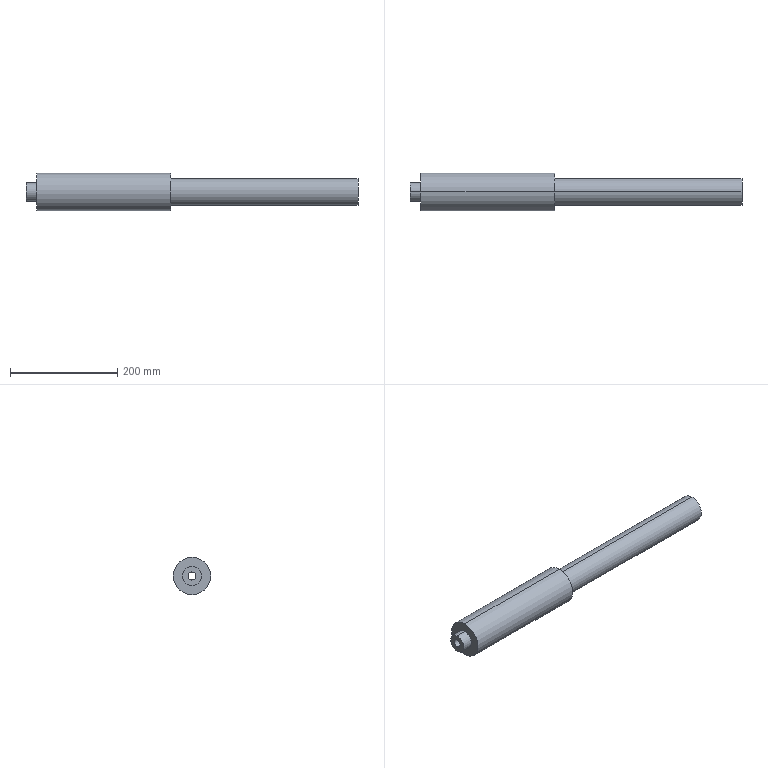Part | SolidWorks | features Revolution 1 | 1 solid | 18 faces | box 620 x 70 x 70 mm | volume 957204 mm3 | cylinder 12 | plane 6 | commonest cylinder face diameters 50 x4 15 x2 30 x2 35 x2 70 x2
STEP:
#1=CARTESIAN_POINT('',(271.174,193.285,-25.));
#2=VERTEX_POINT('',#1);
#3=CARTESIAN_POINT('',(271.174,193.285,25.));
#4=VERTEX_POINT('',#3);
#5=CARTESIAN_POINT('',(271.174,193.285,0.));
#6=DIRECTION('',(-1.,0.,0.));
#7=DIRECTION('',(0.,0.,1.));
#8=AXIS2_PLACEMENT_3D('',#5,#6,#7);
#9=CIRCLE('',#8,25.);
#10=EDGE_CURVE('',#2,#4,#9,.T.);
#11=ORIENTED_EDGE('',*,*,#10,.F.);
#12=CARTESIAN_POINT('',(41.174,193.285,-25.));
#13=VERTEX_POINT('',#12);
#14=CARTESIAN_POINT('',(-12.561,193.285,-25.));
#15=DIRECTION('',(-1.,0.,0.));
#16=VECTOR('',#15,1000.);
#17=LINE('',#14,#16);
#18=EDGE_CURVE('',#2,#13,#17,.T.);
#19=ORIENTED_EDGE('',*,*,#18,.T.);
#20=CARTESIAN_POINT('',(41.174,193.285,25.));
#21=VERTEX_POINT('',#20);
#22=CARTESIAN_POINT('',(41.174,193.285,0.));
#23=DIRECTION('',(-1.,0.,0.));
#24=DIRECTION('',(0.,0.,1.));
#25=AXIS2_PLACEMENT_3D('',#22,#23,#24);
#26=CIRCLE('',#25,25.);
#27=EDGE_CURVE('',#13,#21,#26,.T.);
#28=ORIENTED_EDGE('',*,*,#27,.T.);
#29=CARTESIAN_POINT('',(-12.561,193.285,25.));
#30=DIRECTION('',(-1.,0.,0.));
#31=VECTOR('',#30,1000.);
#32=LINE('',#29,#31);
#33=EDGE_CURVE('',#4,#21,#32,.T.);
#34=ORIENTED_EDGE('',*,*,#33,.F.);
#35=EDGE_LOOP('',(#11,#19,#28,#34));
#36=FACE_OUTER_BOUND('',#35,.T.);
#37=CARTESIAN_POINT('',(-12.561,193.285,0.));
#38=DIRECTION('',(-1.,0.,0.));
#39=DIRECTION('',(0.,0.,1.));
#40=AXIS2_PLACEMENT_3D('',#37,#38,#39);
#41=CYLINDRICAL_SURFACE('',#40,25.);
#42=ADVANCED_FACE('',(#36),#41,.F.);
#43=CARTESIAN_POINT('',(41.174,193.285,-7.5));
#44=VERTEX_POINT('',#43);
#45=CARTESIAN_POINT('',(41.174,193.285,7.5));
#46=VERTEX_POINT('',#45);
#47=CARTESIAN_POINT('',(41.174,193.285,0.));
#48=DIRECTION('',(-1.,0.,0.));
#49=DIRECTION('',(0.,0.,1.));
#50=AXIS2_PLACEMENT_3D('',#47,#48,#49);
#51=CIRCLE('',#50,7.5);
#52=EDGE_CURVE('',#44,#46,#51,.T.);
#53=ORIENTED_EDGE('',*,*,#52,.F.);
#54=CARTESIAN_POINT('',(11.174,193.285,-7.5));
#55=VERTEX_POINT('',#54);
#56=CARTESIAN_POINT('',(-12.561,193.285,-7.5));
#57=DIRECTION('',(-1.,0.,0.));
#58=VECTOR('',#57,1000.);
#59=LINE('',#56,#58);
#60=EDGE_CURVE('',#44,#55,#59,.T.);
#61=ORIENTED_EDGE('',*,*,#60,.T.);
#62=CARTESIAN_POINT('',(11.174,193.285,7.5));
#63=VERTEX_POINT('',#62);
#64=CARTESIAN_POINT('',(11.174,193.285,0.));
#65=DIRECTION('',(-1.,0.,0.));
#66=DIRECTION('',(0.,0.,1.));
#67=AXIS2_PLACEMENT_3D('',#64,#65,#66);
#68=CIRCLE('',#67,7.5);
#69=EDGE_CURVE('',#55,#63,#68,.T.);
#70=ORIENTED_EDGE('',*,*,#69,.T.);
#71=CARTESIAN_POINT('',(-12.561,193.285,7.5));
#72=DIRECTION('',(-1.,0.,0.));
#73=VECTOR('',#72,1000.);
#74=LINE('',#71,#73);
#75=EDGE_CURVE('',#46,#63,#74,.T.);
#76=ORIENTED_EDGE('',*,*,#75,.F.);
#77=EDGE_LOOP('',(#53,#61,#70,#76));
#78=FACE_OUTER_BOUND('',#77,.T.);
#79=CARTESIAN_POINT('',(-12.561,193.285,0.));
#80=DIRECTION('',(-1.,0.,0.));
#81=DIRECTION('',(0.,0.,1.));
#82=AXIS2_PLACEMENT_3D('',#79,#80,#81);
#83=CYLINDRICAL_SURFACE('',#82,7.5);
#84=ADVANCED_FACE('',(#78),#83,.F.);
#85=CARTESIAN_POINT('',(31.174,193.285,17.5));
#86=VERTEX_POINT('',#85);
#87=CARTESIAN_POINT('',(31.174,193.285,-17.5));
#88=VERTEX_POINT('',#87);
#89=CARTESIAN_POINT('',(31.174,193.285,0.));
#90=DIRECTION('',(-1.,0.,0.));
#91=DIRECTION('',(0.,0.,1.));
#92=AXIS2_PLACEMENT_3D('',#89,#90,#91);
#93=CIRCLE('',#92,17.5);
#94=EDGE_CURVE('',#86,#88,#93,.T.);
#95=ORIENTED_EDGE('',*,*,#94,.T.);
#96=CARTESIAN_POINT('',(11.174,193.285,-17.5));
#97=VERTEX_POINT('',#96);
#98=CARTESIAN_POINT('',(-12.561,193.285,-17.5));
#99=DIRECTION('',(-1.,0.,0.));
#100=VECTOR('',#99,1000.);
#101=LINE('',#98,#100);
#102=EDGE_CURVE('',#88,#97,#101,.T.);
#103=ORIENTED_EDGE('',*,*,#102,.T.);
#104=CARTESIAN_POINT('',(11.174,193.285,17.5));
#105=VERTEX_POINT('',#104);
#106=CARTESIAN_POINT('',(11.174,193.285,0.));
#107=DIRECTION('',(-1.,0.,0.));
#108=DIRECTION('',(0.,0.,1.));
#109=AXIS2_PLACEMENT_3D('',#106,#107,#108);
#110=CIRCLE('',#109,17.5);
#111=EDGE_CURVE('',#105,#97,#110,.T.);
#112=ORIENTED_EDGE('',*,*,#111,.F.);
#113=CARTESIAN_POINT('',(-12.561,193.285,17.5));
#114=DIRECTION('',(-1.,0.,0.));
#115=VECTOR('',#114,1000.);
#116=LINE('',#113,#115);
#117=EDGE_CURVE('',#86,#105,#116,.T.);
#118=ORIENTED_EDGE('',*,*,#117,.F.);
#119=EDGE_LOOP('',(#95,#103,#112,#118));
#120=FACE_OUTER_BOUND('',#119,.T.);
#121=CARTESIAN_POINT('',(-12.561,193.285,0.));
#122=DIRECTION('',(-1.,0.,0.));
#123=DIRECTION('',(0.,0.,1.));
#124=AXIS2_PLACEMENT_3D('',#121,#122,#123);
#125=CYLINDRICAL_SURFACE('',#124,17.5);
#126=ADVANCED_FACE('',(#120),#125,.T.);
#127=CARTESIAN_POINT('',(281.174,193.285,35.));
#128=VERTEX_POINT('',#127);
#129=CARTESIAN_POINT('',(281.174,193.285,-35.));
#130=VERTEX_POINT('',#129);
#131=CARTESIAN_POINT('',(281.174,193.285,0.));
#132=DIRECTION('',(-1.,0.,0.));
#133=DIRECTION('',(0.,0.,1.));
#134=AXIS2_PLACEMENT_3D('',#131,#132,#133);
#135=CIRCLE('',#134,35.);
#136=EDGE_CURVE('',#128,#130,#135,.T.);
#137=ORIENTED_EDGE('',*,*,#136,.T.);
#138=CARTESIAN_POINT('',(31.174,193.285,-35.));
#139=VERTEX_POINT('',#138);
#140=CARTESIAN_POINT('',(-12.561,193.285,-35.));
#141=DIRECTION('',(-1.,0.,0.));
#142=VECTOR('',#141,1000.);
#143=LINE('',#140,#142);
#144=EDGE_CURVE('',#130,#139,#143,.T.);
#145=ORIENTED_EDGE('',*,*,#144,.T.);
#146=CARTESIAN_POINT('',(31.174,193.285,35.));
#147=VERTEX_POINT('',#146);
#148=CARTESIAN_POINT('',(31.174,193.285,0.));
#149=DIRECTION('',(-1.,0.,0.));
#150=DIRECTION('',(0.,0.,1.));
#151=AXIS2_PLACEMENT_3D('',#148,#149,#150);
#152=CIRCLE('',#151,35.);
#153=EDGE_CURVE('',#147,#139,#152,.T.);
#154=ORIENTED_EDGE('',*,*,#153,.F.);
#155=CARTESIAN_POINT('',(-12.561,193.285,35.));
#156=DIRECTION('',(-1.,0.,0.));
#157=VECTOR('',#156,1000.);
#158=LINE('',#155,#157);
#159=EDGE_CURVE('',#128,#147,#158,.T.);
#160=ORIENTED_EDGE('',*,*,#159,.F.);
#161=EDGE_LOOP('',(#137,#145,#154,#160));
#162=FACE_OUTER_BOUND('',#161,.T.);
#163=CARTESIAN_POINT('',(-12.561,193.285,0.));
#164=DIRECTION('',(-1.,0.,0.));
#165=DIRECTION('',(0.,0.,1.));
#166=AXIS2_PLACEMENT_3D('',#163,#164,#165);
#167=CYLINDRICAL_SURFACE('',#166,35.);
#168=ADVANCED_FACE('',(#162),#167,.T.);
#169=CARTESIAN_POINT('',(631.174,193.285,25.));
#170=VERTEX_POINT('',#169);
#171=CARTESIAN_POINT('',(631.174,193.285,-25.));
#172=VERTEX_POINT('',#171);
#173=CARTESIAN_POINT('',(631.174,193.285,0.));
#174=DIRECTION('',(-1.,0.,0.));
#175=DIRECTION('',(0.,0.,1.));
#176=AXIS2_PLACEMENT_3D('',#173,#174,#175);
#177=CIRCLE('',#176,25.);
#178=EDGE_CURVE('',#170,#172,#177,.T.);
#179=ORIENTED_EDGE('',*,*,#178,.T.);
#180=CARTESIAN_POINT('',(281.174,193.285,-25.));
#181=VERTEX_POINT('',#180);
#182=CARTESIAN_POINT('',(-12.561,193.285,-25.));
#183=DIRECTION('',(-1.,0.,0.));
#184=VECTOR('',#183,1000.);
#185=LINE('',#182,#184);
#186=EDGE_CURVE('',#172,#181,#185,.T.);
#187=ORIENTED_EDGE('',*,*,#186,.T.);
#188=CARTESIAN_POINT('',(281.174,193.285,25.));
#189=VERTEX_POINT('',#188);
#190=CARTESIAN_POINT('',(281.174,193.285,0.));
#191=DIRECTION('',(-1.,0.,0.));
#192=DIRECTION('',(0.,0.,1.));
#193=AXIS2_PLACEMENT_3D('',#190,#191,#192);
#194=CIRCLE('',#193,25.);
#195=EDGE_CURVE('',#189,#181,#194,.T.);
#196=ORIENTED_EDGE('',*,*,#195,.F.);
#197=CARTESIAN_POINT('',(-12.561,193.285,25.));
#198=DIRECTION('',(-1.,0.,0.));
#199=VECTOR('',#198,1000.);
#200=LINE('',#197,#199);
#201=EDGE_CURVE('',#170,#189,#200,.T.);
#202=ORIENTED_EDGE('',*,*,#201,.F.);
#203=EDGE_LOOP('',(#179,#187,#196,#202));
#204=FACE_OUTER_BOUND('',#203,.T.);
#205=CARTESIAN_POINT('',(-12.561,193.285,0.));
#206=DIRECTION('',(-1.,0.,0.));
#207=DIRECTION('',(0.,0.,1.));
#208=AXIS2_PLACEMENT_3D('',#205,#206,#207);
#209=CYLINDRICAL_SURFACE('',#208,25.);
#210=ADVANCED_FACE('',(#204),#209,.T.);
#211=CARTESIAN_POINT('',(631.174,193.285,-15.));
#212=VERTEX_POINT('',#211);
#213=CARTESIAN_POINT('',(631.174,193.285,15.));
#214=VERTEX_POINT('',#213);
#215=CARTESIAN_POINT('',(631.174,193.285,0.));
#216=DIRECTION('',(-1.,0.,0.));
#217=DIRECTION('',(0.,0.,1.));
#218=AXIS2_PLACEMENT_3D('',#215,#216,#217);
#219=CIRCLE('',#218,15.);
#220=EDGE_CURVE('',#212,#214,#219,.T.);
#221=ORIENTED_EDGE('',*,*,#220,.F.);
#222=CARTESIAN_POINT('',(271.174,193.285,-15.));
#223=VERTEX_POINT('',#222);
#224=CARTESIAN_POINT('',(-12.561,193.285,-15.));
#225=DIRECTION('',(-1.,0.,0.));
#226=VECTOR('',#225,1000.);
#227=LINE('',#224,#226);
#228=EDGE_CURVE('',#212,#223,#227,.T.);
#229=ORIENTED_EDGE('',*,*,#228,.T.);
#230=CARTESIAN_POINT('',(271.174,193.285,15.));
#231=VERTEX_POINT('',#230);
#232=CARTESIAN_POINT('',(271.174,193.285,0.));
#233=DIRECTION('',(-1.,0.,0.));
#234=DIRECTION('',(0.,0.,1.));
#235=AXIS2_PLACEMENT_3D('',#232,#233,#234);
#236=CIRCLE('',#235,15.);
#237=EDGE_CURVE('',#223,#231,#236,.T.);
#238=ORIENTED_EDGE('',*,*,#237,.T.);
#239=CARTESIAN_POINT('',(-12.561,193.285,15.));
#240=DIRECTION('',(-1.,0.,0.));
#241=VECTOR('',#240,1000.);
#242=LINE('',#239,#241);
#243=EDGE_CURVE('',#214,#231,#242,.T.);
#244=ORIENTED_EDGE('',*,*,#243,.F.);
#245=EDGE_LOOP('',(#221,#229,#238,#244));
#246=FACE_OUTER_BOUND('',#245,.T.);
#247=CARTESIAN_POINT('',(-12.561,193.285,0.));
#248=DIRECTION('',(-1.,0.,0.));
#249=DIRECTION('',(0.,0.,1.));
#250=AXIS2_PLACEMENT_3D('',#247,#248,#249);
#251=CYLINDRICAL_SURFACE('',#250,15.);
#252=ADVANCED_FACE('',(#246),#251,.F.);
#253=ORIENTED_EDGE('',*,*,#228,.F.);
#254=CARTESIAN_POINT('',(631.174,193.285,0.));
#255=DIRECTION('',(-1.,0.,0.));
#256=DIRECTION('',(0.,0.,1.));
#257=AXIS2_PLACEMENT_3D('',#254,#255,#256);
#258=CIRCLE('',#257,15.);
#259=EDGE_CURVE('',#214,#212,#258,.T.);
#260=ORIENTED_EDGE('',*,*,#259,.F.);
#261=ORIENTED_EDGE('',*,*,#243,.T.);
#262=CARTESIAN_POINT('',(271.174,193.285,0.));
#263=DIRECTION('',(-1.,0.,0.));
#264=DIRECTION('',(0.,0.,1.));
#265=AXIS2_PLACEMENT_3D('',#262,#263,#264);
#266=CIRCLE('',#265,15.);
#267=EDGE_CURVE('',#231,#223,#266,.T.);
#268=ORIENTED_EDGE('',*,*,#267,.T.);
#269=EDGE_LOOP('',(#253,#260,#261,#268));
#270=FACE_OUTER_BOUND('',#269,.T.);
#271=CARTESIAN_POINT('',(-12.561,193.285,0.));
#272=DIRECTION('',(-1.,0.,0.));
#273=DIRECTION('',(0.,0.,1.));
#274=AXIS2_PLACEMENT_3D('',#271,#272,#273);
#275=CYLINDRICAL_SURFACE('',#274,15.);
#276=ADVANCED_FACE('',(#270),#275,.F.);
#277=ORIENTED_EDGE('',*,*,#178,.F.);
#278=CARTESIAN_POINT('',(631.174,193.285,0.));
#279=DIRECTION('',(-1.,0.,0.));
#280=DIRECTION('',(0.,0.,1.));
#281=AXIS2_PLACEMENT_3D('',#278,#279,#280);
#282=CIRCLE('',#281,25.);
#283=EDGE_CURVE('',#172,#170,#282,.T.);
#284=ORIENTED_EDGE('',*,*,#283,.F.);
#285=EDGE_LOOP('',(#277,#284));
#286=FACE_OUTER_BOUND('',#285,.T.);
#287=ORIENTED_EDGE('',*,*,#259,.T.);
#288=ORIENTED_EDGE('',*,*,#220,.T.);
#289=EDGE_LOOP('',(#287,#288));
#290=FACE_BOUND('',#289,.T.);
#291=CARTESIAN_POINT('',(631.174,208.285,0.));
#292=DIRECTION('',(-1.,0.,0.));
#293=DIRECTION('',(0.,0.,1.));
#294=AXIS2_PLACEMENT_3D('',#291,#292,#293);
#295=PLANE('',#294);
#296=ADVANCED_FACE('',(#286,#290),#295,.F.);
#297=ORIENTED_EDGE('',*,*,#186,.F.);
#298=ORIENTED_EDGE('',*,*,#283,.T.);
#299=ORIENTED_EDGE('',*,*,#201,.T.);
#300=CARTESIAN_POINT('',(281.174,193.285,0.));
#301=DIRECTION('',(-1.,0.,0.));
#302=DIRECTION('',(0.,0.,1.));
#303=AXIS2_PLACEMENT_3D('',#300,#301,#302);
#304=CIRCLE('',#303,25.);
#305=EDGE_CURVE('',#181,#189,#304,.T.);
#306=ORIENTED_EDGE('',*,*,#305,.F.);
#307=EDGE_LOOP('',(#297,#298,#299,#306));
#308=FACE_OUTER_BOUND('',#307,.T.);
#309=CARTESIAN_POINT('',(-12.561,193.285,0.));
#310=DIRECTION('',(-1.,0.,0.));
#311=DIRECTION('',(0.,0.,1.));
#312=AXIS2_PLACEMENT_3D('',#309,#310,#311);
#313=CYLINDRICAL_SURFACE('',#312,25.);
#314=ADVANCED_FACE('',(#308),#313,.T.);
#315=ORIENTED_EDGE('',*,*,#136,.F.);
#316=CARTESIAN_POINT('',(281.174,193.285,0.));
#317=DIRECTION('',(-1.,0.,0.));
#318=DIRECTION('',(0.,0.,1.));
#319=AXIS2_PLACEMENT_3D('',#316,#317,#318);
#320=CIRCLE('',#319,35.);
#321=EDGE_CURVE('',#130,#128,#320,.T.);
#322=ORIENTED_EDGE('',*,*,#321,.F.);
#323=EDGE_LOOP('',(#315,#322));
#324=FACE_OUTER_BOUND('',#323,.T.);
#325=ORIENTED_EDGE('',*,*,#195,.T.);
#326=ORIENTED_EDGE('',*,*,#305,.T.);
#327=EDGE_LOOP('',(#325,#326));
#328=FACE_BOUND('',#327,.T.);
#329=CARTESIAN_POINT('',(281.174,218.285,0.));
#330=DIRECTION('',(-1.,0.,0.));
#331=DIRECTION('',(0.,0.,1.));
#332=AXIS2_PLACEMENT_3D('',#329,#330,#331);
#333=PLANE('',#332);
#334=ADVANCED_FACE('',(#324,#328),#333,.F.);
#335=ORIENTED_EDGE('',*,*,#144,.F.);
#336=ORIENTED_EDGE('',*,*,#321,.T.);
#337=ORIENTED_EDGE('',*,*,#159,.T.);
#338=CARTESIAN_POINT('',(31.174,193.285,0.));
#339=DIRECTION('',(-1.,0.,0.));
#340=DIRECTION('',(0.,0.,1.));
#341=AXIS2_PLACEMENT_3D('',#338,#339,#340);
#342=CIRCLE('',#341,35.);
#343=EDGE_CURVE('',#139,#147,#342,.T.);
#344=ORIENTED_EDGE('',*,*,#343,.F.);
#345=EDGE_LOOP('',(#335,#336,#337,#344));
#346=FACE_OUTER_BOUND('',#345,.T.);
#347=CARTESIAN_POINT('',(-12.561,193.285,0.));
#348=DIRECTION('',(-1.,0.,0.));
#349=DIRECTION('',(0.,0.,1.));
#350=AXIS2_PLACEMENT_3D('',#347,#348,#349);
#351=CYLINDRICAL_SURFACE('',#350,35.);
#352=ADVANCED_FACE('',(#346),#351,.T.);
#353=ORIENTED_EDGE('',*,*,#94,.F.);
#354=CARTESIAN_POINT('',(31.174,193.285,0.));
#355=DIRECTION('',(-1.,0.,0.));
#356=DIRECTION('',(0.,0.,1.));
#357=AXIS2_PLACEMENT_3D('',#354,#355,#356);
#358=CIRCLE('',#357,17.5);
#359=EDGE_CURVE('',#88,#86,#358,.T.);
#360=ORIENTED_EDGE('',*,*,#359,.F.);
#361=EDGE_LOOP('',(#353,#360));
#362=FACE_BOUND('',#361,.T.);
#363=ORIENTED_EDGE('',*,*,#153,.T.);
#364=ORIENTED_EDGE('',*,*,#343,.T.);
#365=EDGE_LOOP('',(#363,#364));
#366=FACE_OUTER_BOUND('',#365,.T.);
#367=CARTESIAN_POINT('',(31.174,228.285,0.));
#368=DIRECTION('',(1.,0.,0.));
#369=DIRECTION('',(0.,0.,-1.));
#370=AXIS2_PLACEMENT_3D('',#367,#368,#369);
#371=PLANE('',#370);
#372=ADVANCED_FACE('',(#362,#366),#371,.F.);
#373=ORIENTED_EDGE('',*,*,#102,.F.);
#374=ORIENTED_EDGE('',*,*,#359,.T.);
#375=ORIENTED_EDGE('',*,*,#117,.T.);
#376=CARTESIAN_POINT('',(11.174,193.285,0.));
#377=DIRECTION('',(-1.,0.,0.));
#378=DIRECTION('',(0.,0.,1.));
#379=AXIS2_PLACEMENT_3D('',#376,#377,#378);
#380=CIRCLE('',#379,17.5);
#381=EDGE_CURVE('',#97,#105,#380,.T.);
#382=ORIENTED_EDGE('',*,*,#381,.F.);
#383=EDGE_LOOP('',(#373,#374,#375,#382));
#384=FACE_OUTER_BOUND('',#383,.T.);
#385=CARTESIAN_POINT('',(-12.561,193.285,0.));
#386=DIRECTION('',(-1.,0.,0.));
#387=DIRECTION('',(0.,0.,1.));
#388=AXIS2_PLACEMENT_3D('',#385,#386,#387);
#389=CYLINDRICAL_SURFACE('',#388,17.5);
#390=ADVANCED_FACE('',(#384),#389,.T.);
#391=CARTESIAN_POINT('',(11.174,193.285,0.));
#392=DIRECTION('',(-1.,0.,0.));
#393=DIRECTION('',(0.,0.,1.));
#394=AXIS2_PLACEMENT_3D('',#391,#392,#393);
#395=CIRCLE('',#394,7.5);
#396=EDGE_CURVE('',#63,#55,#395,.T.);
#397=ORIENTED_EDGE('',*,*,#396,.F.);
#398=ORIENTED_EDGE('',*,*,#69,.F.);
#399=EDGE_LOOP('',(#397,#398));
#400=FACE_BOUND('',#399,.T.);
#401=ORIENTED_EDGE('',*,*,#111,.T.);
#402=ORIENTED_EDGE('',*,*,#381,.T.);
#403=EDGE_LOOP('',(#401,#402));
#404=FACE_OUTER_BOUND('',#403,.T.);
#405=CARTESIAN_POINT('',(11.174,200.785,0.));
#406=DIRECTION('',(1.,0.,0.));
#407=DIRECTION('',(0.,0.,-1.));
#408=AXIS2_PLACEMENT_3D('',#405,#406,#407);
#409=PLANE('',#408);
#410=ADVANCED_FACE('',(#400,#404),#409,.F.);
#411=ORIENTED_EDGE('',*,*,#60,.F.);
#412=CARTESIAN_POINT('',(41.174,193.285,0.));
#413=DIRECTION('',(-1.,0.,0.));
#414=DIRECTION('',(0.,0.,1.));
#415=AXIS2_PLACEMENT_3D('',#412,#413,#414);
#416=CIRCLE('',#415,7.5);
#417=EDGE_CURVE('',#46,#44,#416,.T.);
#418=ORIENTED_EDGE('',*,*,#417,.F.);
#419=ORIENTED_EDGE('',*,*,#75,.T.);
#420=ORIENTED_EDGE('',*,*,#396,.T.);
#421=EDGE_LOOP('',(#411,#418,#419,#420));
#422=FACE_OUTER_BOUND('',#421,.T.);
#423=CARTESIAN_POINT('',(-12.561,193.285,0.));
#424=DIRECTION('',(-1.,0.,0.));
#425=DIRECTION('',(0.,0.,1.));
#426=AXIS2_PLACEMENT_3D('',#423,#424,#425);
#427=CYLINDRICAL_SURFACE('',#426,7.5);
#428=ADVANCED_FACE('',(#422),#427,.F.);
#429=CARTESIAN_POINT('',(41.174,193.285,0.));
#430=DIRECTION('',(-1.,0.,0.));
#431=DIRECTION('',(0.,0.,1.));
#432=AXIS2_PLACEMENT_3D('',#429,#430,#431);
#433=CIRCLE('',#432,25.);
#434=EDGE_CURVE('',#21,#13,#433,.T.);
#435=ORIENTED_EDGE('',*,*,#434,.F.);
#436=ORIENTED_EDGE('',*,*,#27,.F.);
#437=EDGE_LOOP('',(#435,#436));
#438=FACE_OUTER_BOUND('',#437,.T.);
#439=ORIENTED_EDGE('',*,*,#417,.T.);
#440=ORIENTED_EDGE('',*,*,#52,.T.);
#441=EDGE_LOOP('',(#439,#440));
#442=FACE_BOUND('',#441,.T.);
#443=CARTESIAN_POINT('',(41.174,200.785,0.));
#444=DIRECTION('',(-1.,0.,0.));
#445=DIRECTION('',(0.,0.,1.));
#446=AXIS2_PLACEMENT_3D('',#443,#444,#445);
#447=PLANE('',#446);
#448=ADVANCED_FACE('',(#438,#442),#447,.F.);
#449=ORIENTED_EDGE('',*,*,#18,.F.);
#450=CARTESIAN_POINT('',(271.174,193.285,0.));
#451=DIRECTION('',(-1.,0.,0.));
#452=DIRECTION('',(0.,0.,1.));
#453=AXIS2_PLACEMENT_3D('',#450,#451,#452);
#454=CIRCLE('',#453,25.);
#455=EDGE_CURVE('',#4,#2,#454,.T.);
#456=ORIENTED_EDGE('',*,*,#455,.F.);
#457=ORIENTED_EDGE('',*,*,#33,.T.);
#458=ORIENTED_EDGE('',*,*,#434,.T.);
#459=EDGE_LOOP('',(#449,#456,#457,#458));
#460=FACE_OUTER_BOUND('',#459,.T.);
#461=CARTESIAN_POINT('',(-12.561,193.285,0.));
#462=DIRECTION('',(-1.,0.,0.));
#463=DIRECTION('',(0.,0.,1.));
#464=AXIS2_PLACEMENT_3D('',#461,#462,#463);
#465=CYLINDRICAL_SURFACE('',#464,25.);
#466=ADVANCED_FACE('',(#460),#465,.F.);
#467=ORIENTED_EDGE('',*,*,#267,.F.);
#468=ORIENTED_EDGE('',*,*,#237,.F.);
#469=EDGE_LOOP('',(#467,#468));
#470=FACE_BOUND('',#469,.T.);
#471=ORIENTED_EDGE('',*,*,#455,.T.);
#472=ORIENTED_EDGE('',*,*,#10,.T.);
#473=EDGE_LOOP('',(#471,#472));
#474=FACE_OUTER_BOUND('',#473,.T.);
#475=CARTESIAN_POINT('',(271.174,218.285,0.));
#476=DIRECTION('',(1.,0.,0.));
#477=DIRECTION('',(0.,0.,-1.));
#478=AXIS2_PLACEMENT_3D('',#475,#476,#477);
#479=PLANE('',#478);
#480=ADVANCED_FACE('',(#470,#474),#479,.F.);
#481=CLOSED_SHELL('',(#42,#84,#126,#168,#210,#252,#276,#296,#314,#334,#352,#372,#390,#410,#428,#448,#466,#480));
#482=MANIFOLD_SOLID_BREP('',#481);
#483=CARTESIAN_POINT('',(0.,0.,0.));
#484=DIRECTION('',(0.,0.,1.));
#485=DIRECTION('',(1.,0.,0.));
#486=AXIS2_PLACEMENT_3D('',#483,#484,#485);
#487=(LENGTH_UNIT()NAMED_UNIT(*)SI_UNIT(.MILLI.,.METRE.));
#488=UNCERTAINTY_MEASURE_WITH_UNIT(LENGTH_MEASURE(0.00001),#487,'','');
#489=(NAMED_UNIT(*)PLANE_ANGLE_UNIT()SI_UNIT($,.RADIAN.));
#490=(NAMED_UNIT(*)SI_UNIT($,.STERADIAN.)SOLID_ANGLE_UNIT());
#491=(GEOMETRIC_REPRESENTATION_CONTEXT(3)GLOBAL_UNCERTAINTY_ASSIGNED_CONTEXT((#488))GLOBAL_UNIT_ASSIGNED_CONTEXT((#487,#489,#490))REPRESENTATION_CONTEXT('',''));
#492=ADVANCED_BREP_SHAPE_REPRESENTATION('',(#482,#486),#491);